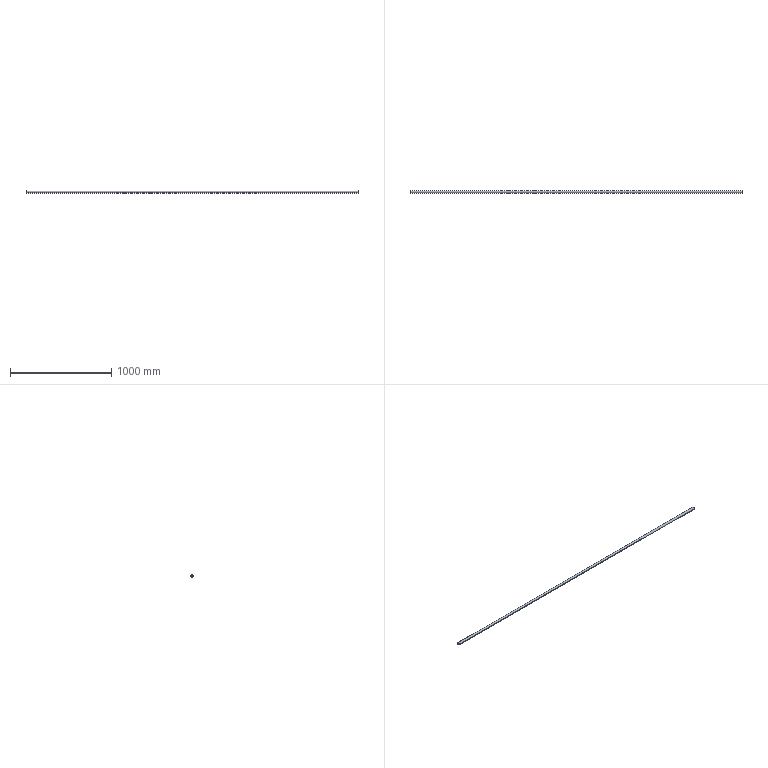Part | STEP file | 粉仓护栏栏杆8_Default<As Machined> | 1 solid | 6 faces | box 3275 x 25 x 25 mm | volume 362677 mm3 | cylinder 4 | plane 2 | commonest cylinder face diameters 22 x2 25 x2
STEP:
#1=CARTESIAN_POINT('',(0.,0.,0.));
#2=DIRECTION('',(0.,0.,1.));
#3=DIRECTION('',(1.,0.,0.));
#4=AXIS2_PLACEMENT_3D('',#1,#2,#3);
#5=CARTESIAN_POINT('',(1637.5,12.5,0.));
#6=VERTEX_POINT('',#5);
#7=CARTESIAN_POINT('',(1637.5,-12.5,0.));
#8=VERTEX_POINT('',#7);
#9=CARTESIAN_POINT('',(1637.5,0.,0.));
#10=DIRECTION('',(1.,0.,0.));
#11=DIRECTION('',(0.,1.,0.));
#12=AXIS2_PLACEMENT_3D('',#9,#10,#11);
#13=CIRCLE('',#12,12.5);
#14=CARTESIAN_POINT('',(1637.5,0.,0.));
#15=DIRECTION('',(-1.,0.,0.));
#16=DIRECTION('',(0.,-1.,0.));
#17=AXIS2_PLACEMENT_3D('',#14,#15,#16);
#18=CYLINDRICAL_SURFACE('',#17,12.5);
#19=CARTESIAN_POINT('',(3.142,0.));
#20=DIRECTION('',(-1.,0.));
#21=VECTOR('',#20,1.);
#22=LINE('',#19,#21);
#23=(GEOMETRIC_REPRESENTATION_CONTEXT(2)PARAMETRIC_REPRESENTATION_CONTEXT()REPRESENTATION_CONTEXT('',''));
#24=DEFINITIONAL_REPRESENTATION('',(#22),#23);
#25=PCURVE('',#18,#24);
#26=CARTESIAN_POINT('',(1637.5,0.,0.));
#27=DIRECTION('',(1.,0.,0.));
#28=DIRECTION('',(0.,1.,0.));
#29=AXIS2_PLACEMENT_3D('',#26,#27,#28);
#30=PLANE('',#29);
#31=CARTESIAN_POINT('',(0.,0.));
#32=DIRECTION('',(1.,0.));
#33=AXIS2_PLACEMENT_2D('',#31,#32);
#34=CIRCLE('',#33,12.5);
#35=(GEOMETRIC_REPRESENTATION_CONTEXT(2)PARAMETRIC_REPRESENTATION_CONTEXT()REPRESENTATION_CONTEXT('',''));
#36=DEFINITIONAL_REPRESENTATION('',(#34),#35);
#37=PCURVE('',#30,#36);
#38=SURFACE_CURVE('',#13,(#25,#37),.PCURVE_S1.);
#39=EDGE_CURVE('',#6,#8,#38,.T.);
#40=ORIENTED_EDGE('',*,*,#39,.F.);
#41=CARTESIAN_POINT('',(-1637.5,12.5,0.));
#42=VERTEX_POINT('',#41);
#43=CARTESIAN_POINT('',(1637.5,12.5,0.));
#44=DIRECTION('',(-1.,0.,0.));
#45=VECTOR('',#44,1.);
#46=LINE('',#43,#45);
#47=CARTESIAN_POINT('',(3.142,0.));
#48=DIRECTION('',(0.,1.));
#49=VECTOR('',#48,1.);
#50=LINE('',#47,#49);
#51=(GEOMETRIC_REPRESENTATION_CONTEXT(2)PARAMETRIC_REPRESENTATION_CONTEXT()REPRESENTATION_CONTEXT('',''));
#52=DEFINITIONAL_REPRESENTATION('',(#50),#51);
#53=PCURVE('',#18,#52);
#54=CARTESIAN_POINT('',(1637.5,0.,0.));
#55=DIRECTION('',(-1.,0.,0.));
#56=DIRECTION('',(0.,-1.,0.));
#57=AXIS2_PLACEMENT_3D('',#54,#55,#56);
#58=CYLINDRICAL_SURFACE('',#57,12.5);
#59=CARTESIAN_POINT('',(3.142,0.));
#60=DIRECTION('',(0.,1.));
#61=VECTOR('',#60,1.);
#62=LINE('',#59,#61);
#63=(GEOMETRIC_REPRESENTATION_CONTEXT(2)PARAMETRIC_REPRESENTATION_CONTEXT()REPRESENTATION_CONTEXT('',''));
#64=DEFINITIONAL_REPRESENTATION('',(#62),#63);
#65=PCURVE('',#58,#64);
#66=SURFACE_CURVE('',#46,(#53,#65),.PCURVE_S1.);
#67=EDGE_CURVE('',#6,#42,#66,.T.);
#68=ORIENTED_EDGE('',*,*,#67,.T.);
#69=CARTESIAN_POINT('',(-1637.5,-12.5,0.));
#70=VERTEX_POINT('',#69);
#71=CARTESIAN_POINT('',(-1637.5,0.,0.));
#72=DIRECTION('',(1.,0.,0.));
#73=DIRECTION('',(0.,1.,0.));
#74=AXIS2_PLACEMENT_3D('',#71,#72,#73);
#75=CIRCLE('',#74,12.5);
#76=CARTESIAN_POINT('',(3.142,3275.));
#77=DIRECTION('',(-1.,0.));
#78=VECTOR('',#77,1.);
#79=LINE('',#76,#78);
#80=(GEOMETRIC_REPRESENTATION_CONTEXT(2)PARAMETRIC_REPRESENTATION_CONTEXT()REPRESENTATION_CONTEXT('',''));
#81=DEFINITIONAL_REPRESENTATION('',(#79),#80);
#82=PCURVE('',#18,#81);
#83=CARTESIAN_POINT('',(-1637.5,0.,0.));
#84=DIRECTION('',(1.,0.,0.));
#85=DIRECTION('',(0.,1.,0.));
#86=AXIS2_PLACEMENT_3D('',#83,#84,#85);
#87=PLANE('',#86);
#88=CARTESIAN_POINT('',(0.,0.));
#89=DIRECTION('',(1.,0.));
#90=AXIS2_PLACEMENT_2D('',#88,#89);
#91=CIRCLE('',#90,12.5);
#92=(GEOMETRIC_REPRESENTATION_CONTEXT(2)PARAMETRIC_REPRESENTATION_CONTEXT()REPRESENTATION_CONTEXT('',''));
#93=DEFINITIONAL_REPRESENTATION('',(#91),#92);
#94=PCURVE('',#87,#93);
#95=SURFACE_CURVE('',#75,(#82,#94),.PCURVE_S1.);
#96=EDGE_CURVE('',#42,#70,#95,.T.);
#97=ORIENTED_EDGE('',*,*,#96,.T.);
#98=CARTESIAN_POINT('',(1637.5,-12.5,0.));
#99=DIRECTION('',(-1.,0.,0.));
#100=VECTOR('',#99,1.);
#101=LINE('',#98,#100);
#102=CARTESIAN_POINT('',(0.,0.));
#103=DIRECTION('',(0.,1.));
#104=VECTOR('',#103,1.);
#105=LINE('',#102,#104);
#106=(GEOMETRIC_REPRESENTATION_CONTEXT(2)PARAMETRIC_REPRESENTATION_CONTEXT()REPRESENTATION_CONTEXT('',''));
#107=DEFINITIONAL_REPRESENTATION('',(#105),#106);
#108=PCURVE('',#18,#107);
#109=CARTESIAN_POINT('',(6.283,0.));
#110=DIRECTION('',(0.,1.));
#111=VECTOR('',#110,1.);
#112=LINE('',#109,#111);
#113=(GEOMETRIC_REPRESENTATION_CONTEXT(2)PARAMETRIC_REPRESENTATION_CONTEXT()REPRESENTATION_CONTEXT('',''));
#114=DEFINITIONAL_REPRESENTATION('',(#112),#113);
#115=PCURVE('',#58,#114);
#116=SURFACE_CURVE('',#101,(#108,#115),.PCURVE_S1.);
#117=EDGE_CURVE('',#8,#70,#116,.T.);
#118=ORIENTED_EDGE('',*,*,#117,.F.);
#119=EDGE_LOOP('',(#40,#68,#97,#118));
#120=FACE_BOUND('',#119,.T.);
#121=ADVANCED_FACE('',(#120),#18,.T.);
#122=CARTESIAN_POINT('',(1637.5,-11.,0.));
#123=VERTEX_POINT('',#122);
#124=CARTESIAN_POINT('',(-1637.5,-11.,0.));
#125=VERTEX_POINT('',#124);
#126=CARTESIAN_POINT('',(1637.5,-11.,0.));
#127=DIRECTION('',(-1.,0.,0.));
#128=VECTOR('',#127,1.);
#129=LINE('',#126,#128);
#130=CARTESIAN_POINT('',(1637.5,0.,0.));
#131=DIRECTION('',(-1.,0.,0.));
#132=DIRECTION('',(0.,-1.,0.));
#133=AXIS2_PLACEMENT_3D('',#130,#131,#132);
#134=CYLINDRICAL_SURFACE('',#133,11.);
#135=CARTESIAN_POINT('',(6.283,0.));
#136=DIRECTION('',(0.,1.));
#137=VECTOR('',#136,1.);
#138=LINE('',#135,#137);
#139=(GEOMETRIC_REPRESENTATION_CONTEXT(2)PARAMETRIC_REPRESENTATION_CONTEXT()REPRESENTATION_CONTEXT('',''));
#140=DEFINITIONAL_REPRESENTATION('',(#138),#139);
#141=PCURVE('',#134,#140);
#142=CARTESIAN_POINT('',(1637.5,0.,0.));
#143=DIRECTION('',(-1.,0.,0.));
#144=DIRECTION('',(0.,-1.,0.));
#145=AXIS2_PLACEMENT_3D('',#142,#143,#144);
#146=CYLINDRICAL_SURFACE('',#145,11.);
#147=CARTESIAN_POINT('',(0.,0.));
#148=DIRECTION('',(0.,1.));
#149=VECTOR('',#148,1.);
#150=LINE('',#147,#149);
#151=(GEOMETRIC_REPRESENTATION_CONTEXT(2)PARAMETRIC_REPRESENTATION_CONTEXT()REPRESENTATION_CONTEXT('',''));
#152=DEFINITIONAL_REPRESENTATION('',(#150),#151);
#153=PCURVE('',#146,#152);
#154=SURFACE_CURVE('',#129,(#141,#153),.PCURVE_S1.);
#155=EDGE_CURVE('',#123,#125,#154,.T.);
#156=ORIENTED_EDGE('',*,*,#155,.T.);
#157=CARTESIAN_POINT('',(-1637.5,11.,0.));
#158=VERTEX_POINT('',#157);
#159=CARTESIAN_POINT('',(-1637.5,0.,0.));
#160=DIRECTION('',(1.,0.,0.));
#161=DIRECTION('',(0.,1.,0.));
#162=AXIS2_PLACEMENT_3D('',#159,#160,#161);
#163=CIRCLE('',#162,11.);
#164=CARTESIAN_POINT('',(9.425,3275.));
#165=DIRECTION('',(-1.,0.));
#166=VECTOR('',#165,1.);
#167=LINE('',#164,#166);
#168=(GEOMETRIC_REPRESENTATION_CONTEXT(2)PARAMETRIC_REPRESENTATION_CONTEXT()REPRESENTATION_CONTEXT('',''));
#169=DEFINITIONAL_REPRESENTATION('',(#167),#168);
#170=PCURVE('',#134,#169);
#171=CARTESIAN_POINT('',(0.,0.));
#172=DIRECTION('',(1.,0.));
#173=AXIS2_PLACEMENT_2D('',#171,#172);
#174=CIRCLE('',#173,11.);
#175=(GEOMETRIC_REPRESENTATION_CONTEXT(2)PARAMETRIC_REPRESENTATION_CONTEXT()REPRESENTATION_CONTEXT('',''));
#176=DEFINITIONAL_REPRESENTATION('',(#174),#175);
#177=PCURVE('',#87,#176);
#178=SURFACE_CURVE('',#163,(#170,#177),.PCURVE_S1.);
#179=EDGE_CURVE('',#125,#158,#178,.T.);
#180=ORIENTED_EDGE('',*,*,#179,.T.);
#181=CARTESIAN_POINT('',(1637.5,11.,0.));
#182=VERTEX_POINT('',#181);
#183=CARTESIAN_POINT('',(1637.5,11.,0.));
#184=DIRECTION('',(-1.,0.,0.));
#185=VECTOR('',#184,1.);
#186=LINE('',#183,#185);
#187=CARTESIAN_POINT('',(3.142,0.));
#188=DIRECTION('',(0.,1.));
#189=VECTOR('',#188,1.);
#190=LINE('',#187,#189);
#191=(GEOMETRIC_REPRESENTATION_CONTEXT(2)PARAMETRIC_REPRESENTATION_CONTEXT()REPRESENTATION_CONTEXT('',''));
#192=DEFINITIONAL_REPRESENTATION('',(#190),#191);
#193=PCURVE('',#134,#192);
#194=CARTESIAN_POINT('',(3.142,0.));
#195=DIRECTION('',(0.,1.));
#196=VECTOR('',#195,1.);
#197=LINE('',#194,#196);
#198=(GEOMETRIC_REPRESENTATION_CONTEXT(2)PARAMETRIC_REPRESENTATION_CONTEXT()REPRESENTATION_CONTEXT('',''));
#199=DEFINITIONAL_REPRESENTATION('',(#197),#198);
#200=PCURVE('',#146,#199);
#201=SURFACE_CURVE('',#186,(#193,#200),.PCURVE_S1.);
#202=EDGE_CURVE('',#182,#158,#201,.T.);
#203=ORIENTED_EDGE('',*,*,#202,.F.);
#204=CARTESIAN_POINT('',(1637.5,0.,0.));
#205=DIRECTION('',(1.,0.,0.));
#206=DIRECTION('',(0.,1.,0.));
#207=AXIS2_PLACEMENT_3D('',#204,#205,#206);
#208=CIRCLE('',#207,11.);
#209=CARTESIAN_POINT('',(9.425,0.));
#210=DIRECTION('',(-1.,0.));
#211=VECTOR('',#210,1.);
#212=LINE('',#209,#211);
#213=(GEOMETRIC_REPRESENTATION_CONTEXT(2)PARAMETRIC_REPRESENTATION_CONTEXT()REPRESENTATION_CONTEXT('',''));
#214=DEFINITIONAL_REPRESENTATION('',(#212),#213);
#215=PCURVE('',#134,#214);
#216=CARTESIAN_POINT('',(0.,0.));
#217=DIRECTION('',(1.,0.));
#218=AXIS2_PLACEMENT_2D('',#216,#217);
#219=CIRCLE('',#218,11.);
#220=(GEOMETRIC_REPRESENTATION_CONTEXT(2)PARAMETRIC_REPRESENTATION_CONTEXT()REPRESENTATION_CONTEXT('',''));
#221=DEFINITIONAL_REPRESENTATION('',(#219),#220);
#222=PCURVE('',#30,#221);
#223=SURFACE_CURVE('',#208,(#215,#222),.PCURVE_S1.);
#224=EDGE_CURVE('',#123,#182,#223,.T.);
#225=ORIENTED_EDGE('',*,*,#224,.F.);
#226=EDGE_LOOP('',(#156,#180,#203,#225));
#227=FACE_BOUND('',#226,.F.);
#228=ADVANCED_FACE('',(#227),#134,.F.);
#229=CARTESIAN_POINT('',(-1637.5,0.,0.));
#230=DIRECTION('',(1.,0.,0.));
#231=DIRECTION('',(0.,1.,0.));
#232=AXIS2_PLACEMENT_3D('',#229,#230,#231);
#233=CIRCLE('',#232,11.);
#234=CARTESIAN_POINT('',(3.142,3275.));
#235=DIRECTION('',(-1.,0.));
#236=VECTOR('',#235,1.);
#237=LINE('',#234,#236);
#238=(GEOMETRIC_REPRESENTATION_CONTEXT(2)PARAMETRIC_REPRESENTATION_CONTEXT()REPRESENTATION_CONTEXT('',''));
#239=DEFINITIONAL_REPRESENTATION('',(#237),#238);
#240=PCURVE('',#146,#239);
#241=CARTESIAN_POINT('',(0.,0.));
#242=DIRECTION('',(1.,0.));
#243=AXIS2_PLACEMENT_2D('',#241,#242);
#244=CIRCLE('',#243,11.);
#245=(GEOMETRIC_REPRESENTATION_CONTEXT(2)PARAMETRIC_REPRESENTATION_CONTEXT()REPRESENTATION_CONTEXT('',''));
#246=DEFINITIONAL_REPRESENTATION('',(#244),#245);
#247=PCURVE('',#87,#246);
#248=SURFACE_CURVE('',#233,(#240,#247),.PCURVE_S1.);
#249=EDGE_CURVE('',#158,#125,#248,.T.);
#250=ORIENTED_EDGE('',*,*,#249,.T.);
#251=ORIENTED_EDGE('',*,*,#155,.F.);
#252=CARTESIAN_POINT('',(1637.5,0.,0.));
#253=DIRECTION('',(1.,0.,0.));
#254=DIRECTION('',(0.,1.,0.));
#255=AXIS2_PLACEMENT_3D('',#252,#253,#254);
#256=CIRCLE('',#255,11.);
#257=CARTESIAN_POINT('',(3.142,0.));
#258=DIRECTION('',(-1.,0.));
#259=VECTOR('',#258,1.);
#260=LINE('',#257,#259);
#261=(GEOMETRIC_REPRESENTATION_CONTEXT(2)PARAMETRIC_REPRESENTATION_CONTEXT()REPRESENTATION_CONTEXT('',''));
#262=DEFINITIONAL_REPRESENTATION('',(#260),#261);
#263=PCURVE('',#146,#262);
#264=CARTESIAN_POINT('',(0.,0.));
#265=DIRECTION('',(1.,0.));
#266=AXIS2_PLACEMENT_2D('',#264,#265);
#267=CIRCLE('',#266,11.);
#268=(GEOMETRIC_REPRESENTATION_CONTEXT(2)PARAMETRIC_REPRESENTATION_CONTEXT()REPRESENTATION_CONTEXT('',''));
#269=DEFINITIONAL_REPRESENTATION('',(#267),#268);
#270=PCURVE('',#30,#269);
#271=SURFACE_CURVE('',#256,(#263,#270),.PCURVE_S1.);
#272=EDGE_CURVE('',#182,#123,#271,.T.);
#273=ORIENTED_EDGE('',*,*,#272,.F.);
#274=ORIENTED_EDGE('',*,*,#202,.T.);
#275=EDGE_LOOP('',(#250,#251,#273,#274));
#276=FACE_BOUND('',#275,.F.);
#277=ADVANCED_FACE('',(#276),#146,.F.);
#278=ORIENTED_EDGE('',*,*,#67,.F.);
#279=CARTESIAN_POINT('',(1637.5,0.,0.));
#280=DIRECTION('',(1.,0.,0.));
#281=DIRECTION('',(0.,1.,0.));
#282=AXIS2_PLACEMENT_3D('',#279,#280,#281);
#283=CIRCLE('',#282,12.5);
#284=CARTESIAN_POINT('',(9.425,0.));
#285=DIRECTION('',(-1.,0.));
#286=VECTOR('',#285,1.);
#287=LINE('',#284,#286);
#288=(GEOMETRIC_REPRESENTATION_CONTEXT(2)PARAMETRIC_REPRESENTATION_CONTEXT()REPRESENTATION_CONTEXT('',''));
#289=DEFINITIONAL_REPRESENTATION('',(#287),#288);
#290=PCURVE('',#58,#289);
#291=CARTESIAN_POINT('',(0.,0.));
#292=DIRECTION('',(1.,0.));
#293=AXIS2_PLACEMENT_2D('',#291,#292);
#294=CIRCLE('',#293,12.5);
#295=(GEOMETRIC_REPRESENTATION_CONTEXT(2)PARAMETRIC_REPRESENTATION_CONTEXT()REPRESENTATION_CONTEXT('',''));
#296=DEFINITIONAL_REPRESENTATION('',(#294),#295);
#297=PCURVE('',#30,#296);
#298=SURFACE_CURVE('',#283,(#290,#297),.PCURVE_S1.);
#299=EDGE_CURVE('',#8,#6,#298,.T.);
#300=ORIENTED_EDGE('',*,*,#299,.F.);
#301=ORIENTED_EDGE('',*,*,#117,.T.);
#302=CARTESIAN_POINT('',(-1637.5,0.,0.));
#303=DIRECTION('',(1.,0.,0.));
#304=DIRECTION('',(0.,1.,0.));
#305=AXIS2_PLACEMENT_3D('',#302,#303,#304);
#306=CIRCLE('',#305,12.5);
#307=CARTESIAN_POINT('',(9.425,3275.));
#308=DIRECTION('',(-1.,0.));
#309=VECTOR('',#308,1.);
#310=LINE('',#307,#309);
#311=(GEOMETRIC_REPRESENTATION_CONTEXT(2)PARAMETRIC_REPRESENTATION_CONTEXT()REPRESENTATION_CONTEXT('',''));
#312=DEFINITIONAL_REPRESENTATION('',(#310),#311);
#313=PCURVE('',#58,#312);
#314=CARTESIAN_POINT('',(0.,0.));
#315=DIRECTION('',(1.,0.));
#316=AXIS2_PLACEMENT_2D('',#314,#315);
#317=CIRCLE('',#316,12.5);
#318=(GEOMETRIC_REPRESENTATION_CONTEXT(2)PARAMETRIC_REPRESENTATION_CONTEXT()REPRESENTATION_CONTEXT('',''));
#319=DEFINITIONAL_REPRESENTATION('',(#317),#318);
#320=PCURVE('',#87,#319);
#321=SURFACE_CURVE('',#306,(#313,#320),.PCURVE_S1.);
#322=EDGE_CURVE('',#70,#42,#321,.T.);
#323=ORIENTED_EDGE('',*,*,#322,.T.);
#324=EDGE_LOOP('',(#278,#300,#301,#323));
#325=FACE_BOUND('',#324,.T.);
#326=ADVANCED_FACE('',(#325),#58,.T.);
#327=ORIENTED_EDGE('',*,*,#224,.F.);
#328=ORIENTED_EDGE('',*,*,#272,.F.);
#329=EDGE_LOOP('',(#327,#328));
#330=FACE_BOUND('',#329,.T.);
#331=ORIENTED_EDGE('',*,*,#299,.T.);
#332=ORIENTED_EDGE('',*,*,#39,.T.);
#333=EDGE_LOOP('',(#331,#332));
#334=FACE_BOUND('',#333,.T.);
#335=ADVANCED_FACE('',(#330,#334),#30,.T.);
#336=ORIENTED_EDGE('',*,*,#179,.T.);
#337=ORIENTED_EDGE('',*,*,#249,.T.);
#338=EDGE_LOOP('',(#336,#337));
#339=FACE_BOUND('',#338,.T.);
#340=ORIENTED_EDGE('',*,*,#322,.F.);
#341=ORIENTED_EDGE('',*,*,#96,.F.);
#342=EDGE_LOOP('',(#340,#341));
#343=FACE_BOUND('',#342,.T.);
#344=ADVANCED_FACE('',(#339,#343),#87,.F.);
#345=CLOSED_SHELL('',(#121,#228,#277,#326,#335,#344));
#346=MANIFOLD_SOLID_BREP('',#345);
#347=(LENGTH_UNIT()NAMED_UNIT(*)SI_UNIT(.MILLI.,.METRE.));
#348=UNCERTAINTY_MEASURE_WITH_UNIT(LENGTH_MEASURE(0.0000001),#347,'','');
#349=(NAMED_UNIT(*)PLANE_ANGLE_UNIT()SI_UNIT($,.RADIAN.));
#350=(NAMED_UNIT(*)SI_UNIT($,.STERADIAN.)SOLID_ANGLE_UNIT());
#351=(GEOMETRIC_REPRESENTATION_CONTEXT(3)GLOBAL_UNCERTAINTY_ASSIGNED_CONTEXT((#348))GLOBAL_UNIT_ASSIGNED_CONTEXT((#347,#349,#350))REPRESENTATION_CONTEXT('',''));
#352=ADVANCED_BREP_SHAPE_REPRESENTATION('',(#4,#346),#351);